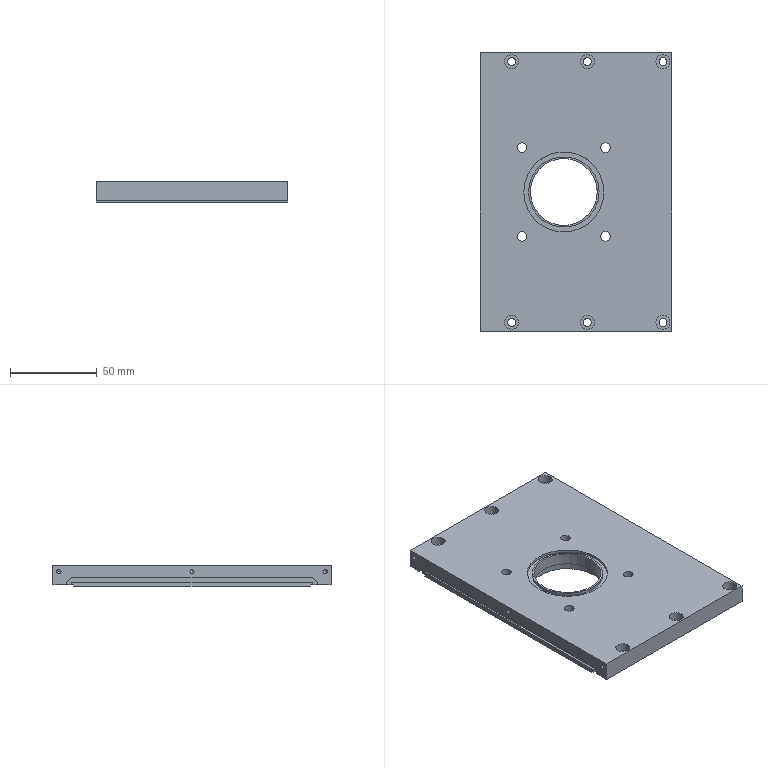NC program | NX | posted with a generic post | part box 110 x 160 x 12 mm
Lines 3477 to 4419 of 4419:
(PLANAR_MILL_COPY_COPY_COPY_COPY_COPY_COPY_1_COPY_1_COPY , TOOL : D6A45)
N6940 T01 M6
N6942 G54
N6944 G17 G0 G90 X-65.933 Y0.483 B0. C0. S9500 M3
N6946 G43 Z30. H1
N6948 Z0.84
N6950 G94 G1 X-66.061 Y0.254 Z0.77 F1250.
N6952 Y-0.254 Z0.634
N6954 X-65.771 Y-0.771 Z0.475
N6956 X-65.254 Y-1.061 Z0.316
N6958 X-64.746 Z0.18
N6960 X-64.229 Y-0.771 Z0.021
N6962 X-63.939 Y-0.254 Z-0.138
N6964 Y0.254 Z-0.274
N6966 X-64.229 Y0.771 Z-0.433
N6968 X-64.746 Y1.061 Z-0.592
N6970 X-65. Z-0.66
N6972 G3 X-66.061 Y0. R1.061
N6974 X-65. Y1.061 R-1.061
N6976 X-65.866 Y0.561 R1.
N6978 G1 Z0.84
N6980 G0 Z30.
N6982 X-44.318 Y1.717
N6984 Z0.84
N6986 G1 Z-0.66
N6988 X-44.134 Y2.44
N6990 G3 X-45. Y2.94 R1.
N6992 G1 X-45.5
N6994 G3 X-47.44 Y1. R1.94
N6996 X-45.5 Y-0.94 R1.94
N6998 G1 X-44.5
N7000 G3 X-42.56 Y1. R1.94
N7002 X-44.5 Y2.94 R1.94
N7004 G1 X-45.
N7006 G3 X-45.866 Y2.44 R1.
N7008 G1 X-45.682 Y1.717
N7010 Z0.84
N7012 G0 Z30.
N7014 X-0.933 Y0.483
N7016 Z0.84
N7018 G1 X-1.061 Y0.254 Z0.77
N7020 Y-0.254 Z0.634
N7022 X-0.771 Y-0.771 Z0.475
N7024 X-0.254 Y-1.061 Z0.316
N7026 X0.254 Z0.18
N7028 X0.771 Y-0.771 Z0.021
N7030 X1.061 Y-0.254 Z-0.138
N7032 Y0.254 Z-0.274
N7034 X0.771 Y0.771 Z-0.433
N7036 X0.254 Y1.061 Z-0.592
N7038 X0. Z-0.66
N7040 G3 X-1.061 Y0. R1.061
N7042 X0. Y1.061 R-1.061
N7044 X-0.866 Y0.561 R1.
N7046 G1 Z0.84
N7048 G0 Z30.
N7050 X45.381 Y1.634
N7052 Z0.84
N7054 G1 Z-0.66
N7056 X45.866 Y2.44
N7058 G3 X45. Y2.94 R1.
N7060 X43.06 Y1. R1.94
N7062 X45. Y2.94 R-1.94
N7064 X44.134 Y2.44 R1.
N7066 G1 X44.619 Y1.634
N7068 Z0.84
N7070 G0 Z30.
N7072 X64.067 Y0.483
N7074 Z0.84
N7076 G1 X63.939 Y0.254 Z0.77
N7078 Y-0.254 Z0.634
N7080 X64.229 Y-0.771 Z0.475
N7082 X64.746 Y-1.061 Z0.316
N7084 X65.254 Z0.18
N7086 X65.771 Y-0.771 Z0.021
N7088 X66.061 Y-0.254 Z-0.138
N7090 Y0.254 Z-0.274
N7092 X65.771 Y0.771 Z-0.433
N7094 X65.254 Y1.061 Z-0.592
N7096 X65. Z-0.66
N7098 G3 X63.939 Y0. R1.061
N7100 X65. Y1.061 R-1.061
N7102 X64.134 Y0.561 R1.
N7104 G1 Z0.84
N7106 G0 Z30.
N7108 M5
(刀补17 , TOOL : D3)
N7110 T17 M6
N7112 G54
N7114 G17 G0 G90 X-46.153 Y1.662 B0. C0. S9500 M3
N7116 G43 Z30. H17
N7118 Z1.
N7120 G94 G1 X-46.234 Y1.591 Z0.994 F1000.
N7122 X-46.392 Y1.304 Z0.977
N7124 X-46.442 Y0.98 Z0.96
N7126 X-46.379 Y0.659 Z0.943
N7128 X-46.209 Y0.379 Z0.926
N7130 X-46.001 Y0.201 Z0.911
N7132 X-45.826 Y0.115 Z0.901
N7134 X-45.637 Y0.067 Z0.891
N7136 X-44.363 Z0.824
N7138 X-44.105 Y0.144 Z0.81
N7140 X-43.879 Y0.291 Z0.796
N7142 X-43.704 Y0.496 Z0.782
N7144 X-43.592 Y0.746 Z0.767
N7146 X-43.559 Y1.063 Z0.751
N7148 X-43.634 Y1.372 Z0.734
N7150 X-43.808 Y1.64 Z0.717
N7152 X-44.06 Y1.834 Z0.701
N7154 X-44.363 Y1.933 Z0.684
N7156 X-45.637 Z0.617
N7158 X-45.735 Y1.913 Z0.612
N7160 X-45.987 Y1.807 Z0.598
N7162 X-46.234 Y1.591 Z0.58
N7164 X-46.392 Y1.304 Z0.563
N7166 X-46.442 Y0.98 Z0.546
N7168 X-46.379 Y0.659 Z0.529
N7170 X-46.209 Y0.379 Z0.512
N7172 X-46.001 Y0.201 Z0.497
N7174 X-45.826 Y0.115 Z0.487
N7176 X-45.637 Y0.067 Z0.477
N7178 X-44.363 Z0.41
N7180 X-44.105 Y0.144 Z0.396
N7182 X-43.879 Y0.291 Z0.382
N7184 X-43.704 Y0.496 Z0.368
N7186 X-43.592 Y0.746 Z0.354
N7188 X-43.559 Y1.063 Z0.337
N7190 X-43.634 Y1.372 Z0.32
N7192 X-43.808 Y1.64 Z0.303
N7194 X-44.06 Y1.834 Z0.287
N7196 X-44.363 Y1.933 Z0.27
N7198 X-45.637 Z0.203
N7200 X-45.735 Y1.913 Z0.198
N7202 X-45.987 Y1.807 Z0.184
N7204 X-46.234 Y1.591 Z0.166
N7206 X-46.392 Y1.304 Z0.149
N7208 X-46.442 Y0.98 Z0.132
N7210 X-46.379 Y0.659 Z0.115
N7212 X-46.209 Y0.379 Z0.098
N7214 X-46.001 Y0.201 Z0.083
N7216 X-45.826 Y0.115 Z0.073
N7218 X-45.637 Y0.067 Z0.063
N7220 X-44.363 Z-0.004
N7222 X-44.105 Y0.144 Z-0.018
N7224 X-43.879 Y0.291 Z-0.032
N7226 X-43.704 Y0.496 Z-0.046
N7228 X-43.592 Y0.746 Z-0.06
N7230 X-43.559 Y1.063 Z-0.077
N7232 X-43.634 Y1.372 Z-0.094
N7234 X-43.808 Y1.64 Z-0.111
N7236 X-44.06 Y1.834 Z-0.127
N7238 X-44.363 Y1.933 Z-0.144
N7240 X-45.637 Z-0.211
N7242 X-45.735 Y1.913 Z-0.216
N7244 X-45.987 Y1.807 Z-0.23
N7246 X-46.234 Y1.591 Z-0.247
N7248 X-46.392 Y1.304 Z-0.265
N7250 X-46.442 Y0.98 Z-0.282
N7252 X-46.379 Y0.659 Z-0.299
N7254 X-46.209 Y0.379 Z-0.316
N7256 X-46.001 Y0.201 Z-0.33
N7258 X-45.826 Y0.115 Z-0.341
N7260 X-45.637 Y0.067 Z-0.351
N7262 X-44.363 Z-0.418
N7264 X-44.105 Y0.144 Z-0.432
N7266 X-43.879 Y0.291 Z-0.446
N7268 X-43.704 Y0.496 Z-0.46
N7270 X-43.592 Y0.746 Z-0.474
N7272 X-43.559 Y1.063 Z-0.491
N7274 X-43.634 Y1.372 Z-0.508
N7276 X-43.808 Y1.64 Z-0.524
N7278 X-44.06 Y1.834 Z-0.541
N7280 X-44.363 Y1.933 Z-0.558
N7282 X-45.637 Z-0.625
N7284 X-45.735 Y1.913 Z-0.63
N7286 X-45.987 Y1.807 Z-0.644
N7288 X-46.234 Y1.591 Z-0.661
N7290 X-46.392 Y1.304 Z-0.679
N7292 X-46.442 Y0.98 Z-0.696
N7294 X-46.379 Y0.659 Z-0.713
N7296 X-46.209 Y0.379 Z-0.73
N7298 X-46.001 Y0.201 Z-0.744
N7300 X-45.826 Y0.115 Z-0.755
N7302 X-45.637 Y0.067 Z-0.765
N7304 X-44.363 Z-0.832
N7306 X-44.105 Y0.144 Z-0.846
N7308 X-43.879 Y0.291 Z-0.86
N7310 X-43.704 Y0.496 Z-0.874
N7312 X-43.592 Y0.746 Z-0.888
N7314 X-43.559 Y1.063 Z-0.905
N7316 X-43.634 Y1.372 Z-0.922
N7318 X-43.808 Y1.64 Z-0.938
N7320 X-44.06 Y1.834 Z-0.955
N7322 X-44.363 Y1.933 Z-0.972
N7324 X-44.902 Z-1.
N7326 G41 X-45. Y1.95 D17
N7328 X-45.5
N7330 G3 X-46.45 Y1. R0.95
N7332 X-45.5 Y0.05 R0.95
N7334 G1 X-44.5
N7336 G3 X-43.55 Y1. R0.95
N7338 X-44.5 Y1.95 R0.95
N7340 G1 X-45.
N7342 X-45.359 Z-1.06
N7344 X-45.478 Y1.946 Z-1.08
N7346 X-45.591 Y1.936 Z-1.099
N7348 X-45.67 Y1.928 Z-1.112
N7350 X-45.713 Y1.916 Z-1.12
N7352 X-45.829 Y1.885 Z-1.14
N7354 X-45.9 Y1.852 Z-1.153
N7356 X-45.935 Y1.835 Z-1.16
N7358 X-46.017 Y1.786 Z-1.176
N7360 X-46.082 Y1.741 Z-1.189
N7362 X-46.129 Y1.701 Z-1.2
N7364 X-46.196 Y1.635 Z-1.216
N7366 X-46.228 Y1.6 Z-1.224
N7368 X-46.283 Y1.521 Z-1.24
N7370 X-46.336 Y1.433 Z-1.257
N7372 X-46.37 Y1.361 Z-1.271
N7374 X-46.39 Y1.31 Z-1.28
N7376 X-46.425 Y1.183 Z-1.302
N7378 X-46.431 Y1.149 Z-1.308
N7380 X-46.438 Y1.079 Z-1.32
N7382 X-46.442 Y0.968 Z-1.339
N7384 X-46.435 Y0.889 Z-1.352
N7386 X-46.431 Y0.842 Z-1.36
N7388 X-46.41 Y0.762 Z-1.374
N7390 X-46.39 Y0.686 Z-1.387
N7392 X-46.359 Y0.617 Z-1.4
N7394 X-46.312 Y0.52 Z-1.418
N7396 X-46.267 Y0.455 Z-1.431
N7398 X-46.238 Y0.414 Z-1.44
N7400 X-46.176 Y0.345 Z-1.456
N7402 X-46.12 Y0.29 Z-1.469
N7404 X-46.068 Y0.25 Z-1.48
N7406 X-45.982 Y0.189 Z-1.498
N7408 X-45.912 Y0.154 Z-1.511
N7410 X-45.863 Y0.132 Z-1.52
N7412 X-45.778 Y0.1 Z-1.535
N7414 X-45.701 Y0.08 Z-1.549
N7416 X-45.636 Y0.068 Z-1.56
N7418 X-45.517 Y0.057 Z-1.58
N7420 X-45.398 Y0.05 Z-1.6
N7422 X-44.681 Z-1.72
N7424 X-44.562 Z-1.74
N7426 X-44.443 Y0.061 Z-1.76
N7428 X-44.328 Y0.073 Z-1.779
N7430 X-44.252 Y0.092 Z-1.793
N7432 X-44.21 Y0.104 Z-1.8
N7434 X-44.122 Y0.138 Z-1.816
N7436 X-44.051 Y0.172 Z-1.829
N7438 X-43.996 Y0.204 Z-1.84
N7440 X-43.917 Y0.259 Z-1.856
N7442 X-43.88 Y0.289 Z-1.864
N7444 X-43.815 Y0.355 Z-1.88
N7446 X-43.748 Y0.434 Z-1.897
N7448 X-43.703 Y0.499 Z-1.911
N7450 X-43.674 Y0.545 Z-1.92
N7452 X-43.621 Y0.658 Z-1.941
N7454 X-43.608 Y0.693 Z-1.947
N7456 X-43.589 Y0.766 Z-1.96
N7458 X-43.566 Y0.882 Z-1.98
N7460 X-43.55 Y1. Z-2.
N7462 G3 X-44.5 Y1.95 R0.95
N7464 G1 X-45.
N7466 X-45.359 Z-2.06
N7468 X-45.478 Y1.946 Z-2.08
N7470 X-45.596 Y1.936 Z-2.1
N7472 X-45.713 Y1.916 Z-2.12
N7474 X-45.803 Y1.893 Z-2.136
N7476 X-45.846 Y1.877 Z-2.143
N7478 X-45.935 Y1.835 Z-2.16
N7480 X-46.016 Y1.787 Z-2.176
N7482 X-46.081 Y1.742 Z-2.189
N7484 X-46.129 Y1.701 Z-2.2
N7486 X-46.197 Y1.633 Z-2.216
N7488 X-46.23 Y1.597 Z-2.224
N7490 X-46.283 Y1.521 Z-2.24
N7492 X-46.336 Y1.432 Z-2.257
N7494 X-46.369 Y1.361 Z-2.271
N7496 X-46.39 Y1.31 Z-2.28
N7498 X-46.414 Y1.226 Z-2.295
N7500 X-46.425 Y1.183 Z-2.302
N7502 X-46.431 Y1.149 Z-2.308
N7504 X-46.437 Y1.079 Z-2.32
N7506 X-46.442 Y0.968 Z-2.339
N7508 X-46.435 Y0.89 Z-2.352
N7510 X-46.43 Y0.842 Z-2.36
N7512 X-46.41 Y0.762 Z-2.374
N7514 X-46.39 Y0.686 Z-2.387
N7516 X-46.359 Y0.617 Z-2.4
N7518 X-46.312 Y0.52 Z-2.418
N7520 X-46.267 Y0.456 Z-2.431
N7522 X-46.238 Y0.414 Z-2.44
N7524 X-46.176 Y0.346 Z-2.455
N7526 X-46.121 Y0.29 Z-2.469
N7528 X-46.068 Y0.25 Z-2.48
N7530 X-45.983 Y0.189 Z-2.498
N7532 X-45.912 Y0.154 Z-2.511
N7534 X-45.863 Y0.132 Z-2.52
N7536 X-45.778 Y0.101 Z-2.535
N7538 X-45.702 Y0.081 Z-2.549
N7540 X-45.636 Y0.068 Z-2.56
N7542 X-45.517 Y0.057 Z-2.58
N7544 X-45.398 Y0.05 Z-2.6
N7546 X-44.681 Z-2.72
N7548 X-44.562 Y0.051 Z-2.74
N7550 X-44.443 Y0.061 Z-2.76
N7552 X-44.328 Y0.073 Z-2.779
N7554 X-44.252 Y0.093 Z-2.793
N7556 X-44.21 Y0.104 Z-2.8
N7558 X-44.123 Y0.138 Z-2.816
N7560 X-44.051 Y0.171 Z-2.829
N7562 X-43.996 Y0.204 Z-2.84
N7564 X-43.918 Y0.259 Z-2.856
N7566 X-43.881 Y0.289 Z-2.864
N7568 X-43.815 Y0.355 Z-2.88
N7570 X-43.748 Y0.434 Z-2.897
N7572 X-43.703 Y0.498 Z-2.911
N7574 X-43.674 Y0.545 Z-2.92
N7576 X-43.621 Y0.661 Z-2.942
N7578 X-43.608 Y0.695 Z-2.948
N7580 X-43.589 Y0.766 Z-2.96
N7582 X-43.566 Y0.882 Z-2.98
N7584 X-43.55 Y1. Z-3.
N7586 G3 X-44.5 Y1.95 R0.95
N7588 G1 X-45.
N7590 X-45.359 Z-3.06
N7592 X-45.478 Y1.946 Z-3.08
N7594 X-45.596 Y1.936 Z-3.1
N7596 X-45.713 Y1.916 Z-3.12
N7598 X-45.802 Y1.893 Z-3.135
N7600 X-45.845 Y1.877 Z-3.143
N7602 X-45.875 Y1.863 Z-3.149
N7604 X-45.935 Y1.835 Z-3.16
N7606 X-46.017 Y1.786 Z-3.176
N7608 X-46.081 Y1.741 Z-3.189
N7610 X-46.129 Y1.7 Z-3.2
N7612 X-46.197 Y1.633 Z-3.216
N7614 X-46.229 Y1.598 Z-3.224
N7616 X-46.248 Y1.573 Z-3.229
N7618 X-46.283 Y1.521 Z-3.24
N7620 X-46.337 Y1.431 Z-3.258
N7622 X-46.37 Y1.359 Z-3.271
N7624 X-46.39 Y1.31 Z-3.28
N7626 X-46.413 Y1.226 Z-3.295
N7628 X-46.425 Y1.184 Z-3.302
N7630 X-46.431 Y1.149 Z-3.308
N7632 X-46.437 Y1.079 Z-3.32
N7634 X-46.441 Y0.969 Z-3.338
N7636 X-46.435 Y0.891 Z-3.352
N7638 X-46.43 Y0.842 Z-3.36
N7640 X-46.41 Y0.763 Z-3.374
N7642 X-46.39 Y0.687 Z-3.387
N7644 X-46.359 Y0.617 Z-3.4
N7646 X-46.313 Y0.521 Z-3.418
N7648 X-46.267 Y0.456 Z-3.431
N7650 X-46.237 Y0.414 Z-3.44
N7652 X-46.177 Y0.347 Z-3.455
N7654 X-46.121 Y0.291 Z-3.469
N7656 X-46.068 Y0.25 Z-3.48
N7658 X-45.983 Y0.19 Z-3.497
N7660 X-45.913 Y0.155 Z-3.511
N7662 X-45.863 Y0.132 Z-3.52
N7664 X-45.779 Y0.101 Z-3.535
N7666 X-45.703 Y0.081 Z-3.548
N7668 X-45.636 Y0.068 Z-3.56
N7670 X-45.517 Y0.057 Z-3.58
N7672 X-45.398 Y0.05 Z-3.6
N7674 X-44.681 Z-3.72
N7676 X-44.562 Y0.051 Z-3.74
N7678 X-44.443 Y0.061 Z-3.76
N7680 X-44.328 Y0.072 Z-3.779
N7682 X-44.252 Y0.093 Z-3.793
N7684 X-44.211 Y0.104 Z-3.8
N7686 X-44.123 Y0.138 Z-3.816
N7688 X-44.052 Y0.171 Z-3.829
N7690 X-43.997 Y0.204 Z-3.84
N7692 X-43.919 Y0.259 Z-3.856
N7694 X-43.882 Y0.288 Z-3.864
N7696 X-43.815 Y0.355 Z-3.88
N7698 X-43.749 Y0.434 Z-3.897
N7700 X-43.703 Y0.498 Z-3.911
N7702 X-43.674 Y0.545 Z-3.92
N7704 X-43.638 Y0.622 Z-3.934
N7706 X-43.608 Y0.695 Z-3.948
N7708 X-43.589 Y0.766 Z-3.96
N7710 X-43.566 Y0.882 Z-3.98
N7712 X-43.55 Y1. Z-4.
N7714 G3 X-44.5 Y1.95 R0.95
N7716 G1 X-45.
N7718 X-45.359 Z-4.06
N7720 X-45.478 Y1.945 Z-4.08
N7722 X-45.596 Y1.936 Z-4.1
N7724 X-45.713 Y1.916 Z-4.12
N7726 X-45.802 Y1.893 Z-4.135
N7728 X-45.845 Y1.877 Z-4.143
N7730 X-45.935 Y1.835 Z-4.16
N7732 X-46.017 Y1.786 Z-4.176
N7734 X-46.081 Y1.741 Z-4.189
N7736 X-46.129 Y1.7 Z-4.2
N7738 X-46.196 Y1.633 Z-4.216
N7740 X-46.228 Y1.598 Z-4.224
N7742 X-46.247 Y1.573 Z-4.229
N7744 X-46.283 Y1.521 Z-4.24
N7746 X-46.336 Y1.431 Z-4.258
N7748 X-46.37 Y1.36 Z-4.271
N7750 X-46.39 Y1.31 Z-4.28
N7752 X-46.413 Y1.227 Z-4.295
N7754 X-46.424 Y1.185 Z-4.302
N7756 X-46.431 Y1.15 Z-4.308
N7758 X-46.437 Y1.079 Z-4.32
N7760 X-46.441 Y0.97 Z-4.338
N7762 X-46.434 Y0.891 Z-4.352
N7764 X-46.43 Y0.842 Z-4.36
N7766 X-46.41 Y0.764 Z-4.374
N7768 X-46.39 Y0.687 Z-4.387
N7770 X-46.359 Y0.617 Z-4.4
N7772 X-46.313 Y0.521 Z-4.418
N7774 X-46.267 Y0.457 Z-4.431
N7776 X-46.237 Y0.415 Z-4.44
N7778 X-46.177 Y0.347 Z-4.455
N7780 X-46.121 Y0.291 Z-4.469
N7782 X-46.068 Y0.25 Z-4.48
N7784 X-45.984 Y0.19 Z-4.497
N7786 X-45.913 Y0.155 Z-4.511
N7788 X-45.863 Y0.132 Z-4.52
N7790 X-45.78 Y0.101 Z-4.535
N7792 X-45.704 Y0.081 Z-4.548
N7794 X-45.636 Y0.068 Z-4.56
N7796 X-45.517 Y0.057 Z-4.58
N7798 X-45.398 Y0.05 Z-4.6
N7800 X-44.681 Z-4.72
N7802 X-44.562 Y0.051 Z-4.74
N7804 X-44.443 Y0.061 Z-4.76
N7806 X-44.328 Y0.073 Z-4.779
N7808 X-44.252 Y0.093 Z-4.793
N7810 X-44.211 Y0.104 Z-4.8
N7812 X-44.122 Y0.139 Z-4.816
N7814 X-44.05 Y0.172 Z-4.829
N7816 X-43.997 Y0.204 Z-4.84
N7818 X-43.917 Y0.261 Z-4.856
N7820 X-43.879 Y0.291 Z-4.865
N7822 X-43.857 Y0.312 Z-4.87
N7824 X-43.815 Y0.356 Z-4.88
N7826 X-43.748 Y0.435 Z-4.898
N7828 X-43.702 Y0.5 Z-4.911
N7830 X-43.674 Y0.545 Z-4.92
N7832 X-43.639 Y0.621 Z-4.934
N7834 X-43.621 Y0.66 Z-4.941
N7836 X-43.609 Y0.694 Z-4.948
N7838 X-43.589 Y0.766 Z-4.96
N7840 X-43.566 Y0.883 Z-4.98
N7842 X-43.55 Y1. Z-5.
N7844 G3 X-44.5 Y1.95 R0.95
N7846 G1 X-45.
N7848 X-45.359 Z-5.06
N7850 X-45.478 Y1.945 Z-5.08
N7852 X-45.596 Y1.935 Z-5.1
N7854 X-45.713 Y1.916 Z-5.12
N7856 X-45.802 Y1.893 Z-5.135
N7858 X-45.845 Y1.877 Z-5.143
N7860 X-45.935 Y1.835 Z-5.16
N7862 X-46.017 Y1.786 Z-5.176
N7864 X-46.081 Y1.741 Z-5.189
N7866 X-46.129 Y1.7 Z-5.2
N7868 X-46.196 Y1.633 Z-5.216
N7870 X-46.229 Y1.599 Z-5.224
N7872 X-46.283 Y1.521 Z-5.24
N7874 X-46.336 Y1.431 Z-5.258
N7876 X-46.37 Y1.36 Z-5.271
N7878 X-46.39 Y1.31 Z-5.28
N7880 X-46.414 Y1.225 Z-5.295
N7882 X-46.425 Y1.182 Z-5.302
N7884 X-46.431 Y1.148 Z-5.308
N7886 X-46.437 Y1.079 Z-5.32
N7888 X-46.441 Y0.967 Z-5.339
N7890 X-46.434 Y0.889 Z-5.352
N7892 X-46.43 Y0.842 Z-5.36
N7894 X-46.41 Y0.764 Z-5.374
N7896 X-46.39 Y0.688 Z-5.387
N7898 X-46.359 Y0.617 Z-5.4
N7900 X-46.313 Y0.522 Z-5.418
N7902 X-46.268 Y0.457 Z-5.431
N7904 X-46.237 Y0.415 Z-5.44
N7906 X-46.175 Y0.346 Z-5.456
N7908 X-46.119 Y0.29 Z-5.469
N7910 X-46.068 Y0.25 Z-5.48
N7912 X-45.984 Y0.191 Z-5.497
N7914 X-45.913 Y0.156 Z-5.511
N7916 X-45.863 Y0.133 Z-5.52
N7918 X-45.78 Y0.102 Z-5.535
N7920 X-45.704 Y0.081 Z-5.548
N7922 X-45.636 Y0.069 Z-5.56
N7924 X-45.517 Y0.058 Z-5.58
N7926 X-45.398 Y0.05 Z-5.6
N7928 X-44.681 Z-5.72
N7930 X-44.562 Y0.051 Z-5.74
N7932 X-44.443 Y0.061 Z-5.76
N7934 X-44.328 Y0.073 Z-5.779
N7936 X-44.252 Y0.093 Z-5.793
N7938 X-44.211 Y0.104 Z-5.8
N7940 X-44.122 Y0.138 Z-5.816
N7942 X-44.051 Y0.172 Z-5.829
N7944 X-43.997 Y0.205 Z-5.84
N7946 X-43.918 Y0.261 Z-5.856
N7948 X-43.88 Y0.291 Z-5.865
N7950 X-43.858 Y0.312 Z-5.87
N7952 X-43.815 Y0.356 Z-5.88
N7954 X-43.748 Y0.435 Z-5.897
N7956 X-43.703 Y0.499 Z-5.911
N7958 X-43.675 Y0.546 Z-5.92
N7960 X-43.639 Y0.621 Z-5.934
N7962 X-43.621 Y0.659 Z-5.941
N7964 X-43.609 Y0.694 Z-5.947
N7966 X-43.589 Y0.766 Z-5.96
N7968 X-43.567 Y0.883 Z-5.98
N7970 X-43.55 Y1. Z-6.
N7972 G3 X-44.5 Y1.95 R0.95
N7974 G1 X-45.5
N7976 G3 X-46.45 Y1. R0.95
N7978 X-45.5 Y0.05 R0.95
N7980 G1 X-44.5
N7982 G3 X-43.55 Y1. R0.95
N7984 G40
N7986 G1 X-43.567 Y1.098
N7988 Z-5.
N7990 G0 Z30.
N7992 X45.252 Y0.094
N7994 Z1.
N7996 G1 X45.552 Y0.229 Z0.983
N7998 X45.807 Y0.502 Z0.963
N8000 X45.915 Y0.755 Z0.949
N8002 X45.948 Y0.987 Z0.937
N8004 X45.912 Y1.259 Z0.922
N8006 X45.769 Y1.554 Z0.905
N8008 X45.534 Y1.783 Z0.888
N8010 X45.235 Y1.918 Z0.871
N8012 X45.049 Y1.938 Z0.861
N8014 X44.863 Z0.851
N8016 X44.758 Y1.916 Z0.845
N8018 X44.505 Y1.808 Z0.831
N8020 X44.26 Y1.592 Z0.814
N8022 X44.103 Y1.305 Z0.797
N8024 X44.052 Y0.982 Z0.78
N8026 X44.115 Y0.661 Z0.762
N8028 X44.283 Y0.38 Z0.745
N8030 X44.49 Y0.201 Z0.731
N8032 X44.839 Y0.066 Z0.711
N8034 X45.212 Y0.076 Z0.692
N8036 X45.552 Y0.229 Z0.672
N8038 X45.807 Y0.502 Z0.653
N8040 X45.915 Y0.755 Z0.638
N8042 X45.948 Y0.987 Z0.626
N8044 X45.912 Y1.259 Z0.612
N8046 X45.769 Y1.554 Z0.594
N8048 X45.534 Y1.783 Z0.577
N8050 X45.235 Y1.918 Z0.56
N8052 X45.049 Y1.938 Z0.55
N8054 X44.863 Z0.54
N8056 X44.758 Y1.916 Z0.535
N8058 X44.505 Y1.808 Z0.52
N8060 X44.26 Y1.592 Z0.503
N8062 X44.103 Y1.305 Z0.486
N8064 X44.052 Y0.982 Z0.469
N8066 X44.115 Y0.661 Z0.452
N8068 X44.283 Y0.38 Z0.435
N8070 X44.49 Y0.201 Z0.42
N8072 X44.839 Y0.066 Z0.401
N8074 X45.212 Y0.076 Z0.381
N8076 X45.552 Y0.229 Z0.362
N8078 X45.807 Y0.502 Z0.342
N8080 X45.915 Y0.755 Z0.328
N8082 X45.948 Y0.987 Z0.315
N8084 X45.912 Y1.259 Z0.301
N8086 X45.769 Y1.554 Z0.284
N8088 X45.534 Y1.783 Z0.267
N8090 X45.235 Y1.918 Z0.249
N8092 X45.049 Y1.938 Z0.24
N8094 X44.863 Z0.23
N8096 X44.758 Y1.916 Z0.224
N8098 X44.505 Y1.808 Z0.21
N8100 X44.26 Y1.592 Z0.193
N8102 X44.103 Y1.305 Z0.176
N8104 X44.052 Y0.982 Z0.158
N8106 X44.115 Y0.661 Z0.141
N8108 X44.283 Y0.38 Z0.124
N8110 X44.49 Y0.201 Z0.11
N8112 X44.839 Y0.066 Z0.09
N8114 X45.212 Y0.076 Z0.071
N8116 X45.552 Y0.229 Z0.051
N8118 X45.807 Y0.502 Z0.032
N8120 X45.915 Y0.755 Z0.017
N8122 X45.948 Y0.987 Z0.005
N8124 X45.912 Y1.259 Z-0.01
N8126 X45.769 Y1.554 Z-0.027
N8128 X45.534 Y1.783 Z-0.044
N8130 X45.235 Y1.918 Z-0.061
N8132 X45.049 Y1.938 Z-0.071
N8134 X44.863 Z-0.081
N8136 X44.758 Y1.916 Z-0.086
N8138 X44.505 Y1.808 Z-0.101
N8140 X44.26 Y1.592 Z-0.118
N8142 X44.103 Y1.305 Z-0.135
N8144 X44.052 Y0.982 Z-0.152
N8146 X44.115 Y0.661 Z-0.169
N8148 X44.283 Y0.38 Z-0.186
N8150 X44.49 Y0.201 Z-0.201
N8152 X44.839 Y0.066 Z-0.22
N8154 X45.212 Y0.076 Z-0.24
N8156 X45.552 Y0.229 Z-0.259
N8158 X45.807 Y0.502 Z-0.279
N8160 X45.915 Y0.755 Z-0.293
N8162 X45.948 Y0.987 Z-0.306
N8164 X45.912 Y1.259 Z-0.32
N8166 X45.769 Y1.554 Z-0.337
N8168 X45.534 Y1.783 Z-0.354
N8170 X45.235 Y1.918 Z-0.372
N8172 X45.049 Y1.938 Z-0.381
N8174 X44.863 Z-0.391
N8176 X44.758 Y1.916 Z-0.397
N8178 X44.505 Y1.808 Z-0.411
N8180 X44.26 Y1.592 Z-0.428
N8182 X44.103 Y1.305 Z-0.446
N8184 X44.052 Y0.982 Z-0.463
N8186 X44.115 Y0.661 Z-0.48
N8188 X44.283 Y0.38 Z-0.497
N8190 X44.49 Y0.201 Z-0.511
N8192 X44.839 Y0.066 Z-0.531
N8194 X45.212 Y0.076 Z-0.55
N8196 X45.552 Y0.229 Z-0.57
N8198 X45.807 Y0.502 Z-0.59
N8200 X45.915 Y0.755 Z-0.604
N8202 X45.948 Y0.987 Z-0.616
N8204 X45.912 Y1.259 Z-0.631
N8206 X45.769 Y1.554 Z-0.648
N8208 X45.534 Y1.783 Z-0.665
N8210 X45.235 Y1.918 Z-0.682
N8212 X45.049 Y1.938 Z-0.692
N8214 X44.863 Z-0.702
N8216 X44.758 Y1.916 Z-0.707
N8218 X44.505 Y1.808 Z-0.722
N8220 X44.26 Y1.592 Z-0.739
N8222 X44.103 Y1.305 Z-0.756
N8224 X44.052 Y0.982 Z-0.773
N8226 X44.115 Y0.661 Z-0.79
N8228 X44.283 Y0.38 Z-0.808
N8230 X44.49 Y0.201 Z-0.822
N8232 X44.839 Y0.066 Z-0.841
N8234 X45.212 Y0.076 Z-0.861
N8236 X45.552 Y0.229 Z-0.881
N8238 X45.807 Y0.502 Z-0.9
N8240 X45.915 Y0.755 Z-0.915
N8242 X45.948 Y0.987 Z-0.927
N8244 X45.912 Y1.259 Z-0.941
N8246 X45.769 Y1.554 Z-0.958
N8248 X45.534 Y1.783 Z-0.976
N8250 X45.235 Y1.918 Z-0.993
N8252 X45.098 Y1.933 Z-1.
N8254 G41 X45. Y1.95
N8256 G3 X44.05 Y1. R0.95
N8258 X45. Y1.95 R-0.95
N8260 G1 X44.909 Y1.936 Z-1.021
N8262 X44.827 Y1.928 Z-1.039
N8264 X44.756 Y1.909 Z-1.056
N8266 X44.646 Y1.873 Z-1.082
N8268 X44.571 Y1.838 Z-1.1
N8270 X44.528 Y1.817 Z-1.111
N8272 X44.457 Y1.768 Z-1.131
N8274 X44.39 Y1.721 Z-1.149
N8276 X44.335 Y1.665 Z-1.167
N8278 X44.257 Y1.579 Z-1.193
N8280 X44.21 Y1.512 Z-1.211
N8282 X44.183 Y1.472 Z-1.222
N8284 X44.146 Y1.394 Z-1.242
N8286 X44.111 Y1.319 Z-1.26
N8288 X44.091 Y1.244 Z-1.278
N8290 X44.067 Y1.13 Z-1.304
N8292 X44.06 Y1.048 Z-1.322
N8294 X44.056 Y1. Z-1.333
N8296 X44.064 Y0.914 Z-1.353
N8298 X44.071 Y0.832 Z-1.371
N8300 X44.091 Y0.756 Z-1.389
N8302 X44.127 Y0.646 Z-1.415
N8304 X44.162 Y0.572 Z-1.433
N8306 X44.183 Y0.528 Z-1.444
N8308 X44.232 Y0.457 Z-1.464
N8310 X44.279 Y0.39 Z-1.482
N8312 X44.335 Y0.335 Z-1.5
N8314 X44.421 Y0.257 Z-1.526
N8316 X44.488 Y0.21 Z-1.545
N8318 X44.528 Y0.183 Z-1.556
N8320 X44.606 Y0.146 Z-1.575
N8322 X44.681 Y0.111 Z-1.594
N8324 X44.756 Y0.091 Z-1.611
N8326 X44.87 Y0.067 Z-1.637
N8328 X44.952 Y0.06 Z-1.656
N8330 X45. Y0.056 Z-1.667
N8332 X45.086 Y0.064 Z-1.686
N8334 X45.168 Y0.071 Z-1.705
N8336 X45.244 Y0.091 Z-1.722
N8338 X45.354 Y0.127 Z-1.748
N8340 X45.428 Y0.162 Z-1.767
N8342 X45.472 Y0.183 Z-1.778
N8344 X45.543 Y0.232 Z-1.797
N8346 X45.61 Y0.279 Z-1.816
N8348 X45.665 Y0.335 Z-1.833
N8350 X45.743 Y0.421 Z-1.859
N8352 X45.79 Y0.488 Z-1.878
N8354 X45.817 Y0.528 Z-1.889
N8356 X45.852 Y0.602 Z-1.907
N8358 X45.887 Y0.676 Z-1.926
N8360 X45.909 Y0.757 Z-1.944
N8362 X45.934 Y0.878 Z-1.972
N8364 X45.95 Y1. Z-2.
N8366 G3 X45. Y1.95 R0.95
N8368 G1 X44.909 Y1.936 Z-2.021
N8370 X44.827 Y1.928 Z-2.039
N8372 X44.757 Y1.909 Z-2.056
N8374 X44.646 Y1.873 Z-2.082
N8376 X44.572 Y1.838 Z-2.1
N8378 X44.528 Y1.817 Z-2.111
N8380 X44.458 Y1.768 Z-2.13
N8382 X44.39 Y1.721 Z-2.149
N8384 X44.335 Y1.665 Z-2.167
N8386 X44.257 Y1.579 Z-2.193
N8388 X44.21 Y1.512 Z-2.211
N8390 X44.183 Y1.472 Z-2.222
N8392 X44.146 Y1.394 Z-2.242
N8394 X44.112 Y1.319 Z-2.26
N8396 X44.091 Y1.243 Z-2.278
N8398 X44.067 Y1.13 Z-2.304
N8400 X44.06 Y1.049 Z-2.322
N8402 X44.056 Y1. Z-2.333
N8404 X44.064 Y0.914 Z-2.353
N8406 X44.071 Y0.833 Z-2.371
N8408 X44.091 Y0.757 Z-2.389
N8410 X44.127 Y0.646 Z-2.415
N8412 X44.162 Y0.572 Z-2.433
N8414 X44.183 Y0.528 Z-2.444
N8416 X44.232 Y0.458 Z-2.464
N8418 X44.279 Y0.391 Z-2.482
N8420 X44.335 Y0.335 Z-2.5
N8422 X44.421 Y0.257 Z-2.526
N8424 X44.488 Y0.21 Z-2.544
N8426 X44.528 Y0.183 Z-2.556
N8428 X44.606 Y0.146 Z-2.575
N8430 X44.68 Y0.112 Z-2.593
N8432 X44.757 Y0.091 Z-2.611
N8434 X44.87 Y0.067 Z-2.637
N8436 X44.951 Y0.06 Z-2.656
N8438 X45. Y0.056 Z-2.667
N8440 X45.085 Y0.064 Z-2.686
N8442 X45.167 Y0.071 Z-2.705
N8444 X45.243 Y0.091 Z-2.722
N8446 X45.354 Y0.127 Z-2.748
N8448 X45.428 Y0.162 Z-2.767
N8450 X45.472 Y0.183 Z-2.778
N8452 X45.542 Y0.232 Z-2.797
N8454 X45.609 Y0.279 Z-2.816
N8456 X45.665 Y0.335 Z-2.833
N8458 X45.743 Y0.421 Z-2.859
N8460 X45.789 Y0.488 Z-2.878
N8462 X45.817 Y0.528 Z-2.889
N8464 X45.852 Y0.601 Z-2.907
N8466 X45.886 Y0.676 Z-2.926
N8468 X45.909 Y0.757 Z-2.944
N8470 X45.933 Y0.878 Z-2.972
N8472 X45.95 Y1. Z-3.
N8474 G3 X45. Y1.95 R0.95
N8476 G1 X44.909 Y1.937 Z-3.021
N8478 X44.827 Y1.927 Z-3.039
N8480 X44.757 Y1.909 Z-3.056
N8482 X44.646 Y1.873 Z-3.081
N8484 X44.572 Y1.838 Z-3.1
N8486 X44.528 Y1.817 Z-3.111
N8488 X44.458 Y1.768 Z-3.13
N8490 X44.391 Y1.721 Z-3.149
N8492 X44.335 Y1.665 Z-3.167
N8494 X44.257 Y1.58 Z-3.193
N8496 X44.211 Y1.512 Z-3.211
N8498 X44.183 Y1.472 Z-3.222
N8500 X44.147 Y1.394 Z-3.241
N8502 X44.112 Y1.32 Z-3.26
N8504 X44.091 Y1.243 Z-3.278
N8506 X44.067 Y1.131 Z-3.304
N8508 X44.06 Y1.049 Z-3.322
N8510 X44.056 Y1. Z-3.333
N8512 X44.064 Y0.915 Z-3.353
N8514 X44.071 Y0.833 Z-3.371
N8516 X44.091 Y0.757 Z-3.389
N8518 X44.127 Y0.647 Z-3.415
N8520 X44.162 Y0.573 Z-3.433
N8522 X44.183 Y0.528 Z-3.444
N8524 X44.232 Y0.458 Z-3.464
N8526 X44.279 Y0.391 Z-3.482
N8528 X44.335 Y0.335 Z-3.5
N8530 X44.42 Y0.258 Z-3.526
N8532 X44.488 Y0.211 Z-3.544
N8534 X44.528 Y0.183 Z-3.556
N8536 X44.605 Y0.147 Z-3.575
N8538 X44.68 Y0.112 Z-3.593
N8540 X44.757 Y0.091 Z-3.611
N8542 X44.869 Y0.067 Z-3.637
N8544 X44.951 Y0.06 Z-3.655
N8546 X45. Y0.057 Z-3.667
N8548 X45.085 Y0.064 Z-3.686
N8550 X45.167 Y0.071 Z-3.704
N8552 X45.243 Y0.091 Z-3.722
N8554 X45.353 Y0.127 Z-3.748
N8556 X45.427 Y0.162 Z-3.767
N8558 X45.472 Y0.183 Z-3.778
N8560 X45.541 Y0.232 Z-3.797
N8562 X45.609 Y0.279 Z-3.815
N8564 X45.665 Y0.335 Z-3.833
N8566 X45.742 Y0.42 Z-3.859
N8568 X45.789 Y0.487 Z-3.878
N8570 X45.817 Y0.528 Z-3.889
N8572 X45.851 Y0.601 Z-3.907
N8574 X45.886 Y0.675 Z-3.926
N8576 X45.908 Y0.757 Z-3.944
N8578 X45.933 Y0.878 Z-3.972
N8580 X45.95 Y1. Z-4.
N8582 G3 X45. Y1.95 R0.95
N8584 G1 X44.864 Y1.932 Z-4.031
N8586 X44.827 Y1.927 Z-4.039
N8588 X44.757 Y1.908 Z-4.056
N8590 X44.647 Y1.873 Z-4.081
N8592 X44.573 Y1.838 Z-4.1
N8594 X44.528 Y1.817 Z-4.111
N8596 X44.459 Y1.768 Z-4.13
N8598 X44.391 Y1.721 Z-4.149
N8600 X44.335 Y1.665 Z-4.167
N8602 X44.258 Y1.58 Z-4.192
N8604 X44.211 Y1.513 Z-4.211
N8606 X44.183 Y1.472 Z-4.222
N8608 X44.147 Y1.395 Z-4.241
N8610 X44.112 Y1.32 Z-4.26
N8612 X44.092 Y1.243 Z-4.278
N8614 X44.067 Y1.131 Z-4.304
N8616 X44.061 Y1.05 Z-4.322
N8618 X44.057 Y1. Z-4.333
N8620 X44.064 Y0.916 Z-4.352
N8622 X44.071 Y0.834 Z-4.371
N8624 X44.092 Y0.757 Z-4.389
N8626 X44.127 Y0.647 Z-4.415
N8628 X44.162 Y0.573 Z-4.433
N8630 X44.183 Y0.528 Z-4.444
N8632 X44.231 Y0.458 Z-4.464
N8634 X44.279 Y0.392 Z-4.482
N8636 X44.335 Y0.335 Z-4.5
N8638 X44.42 Y0.258 Z-4.526
N8640 X44.487 Y0.211 Z-4.544
N8642 X44.528 Y0.183 Z-4.556
N8644 X44.605 Y0.146 Z-4.575
N8646 X44.68 Y0.113 Z-4.593
N8648 X44.757 Y0.092 Z-4.611
N8650 X44.869 Y0.068 Z-4.637
N8652 X44.95 Y0.061 Z-4.655
N8654 X45. Y0.057 Z-4.667
N8656 X45.084 Y0.063 Z-4.686
N8658 X45.166 Y0.071 Z-4.704
N8660 X45.243 Y0.092 Z-4.722
N8662 X45.352 Y0.127 Z-4.748
N8664 X45.427 Y0.162 Z-4.766
N8666 X45.472 Y0.183 Z-4.778
N8668 X45.542 Y0.231 Z-4.797
N8670 X45.609 Y0.278 Z-4.815
N8672 X45.665 Y0.335 Z-4.833
N8674 X45.743 Y0.422 Z-4.86
N8676 X45.79 Y0.489 Z-4.878
N8678 X45.817 Y0.528 Z-4.889
N8680 X45.851 Y0.6 Z-4.907
N8682 X45.886 Y0.675 Z-4.925
N8684 X45.908 Y0.757 Z-4.944
N8686 X45.933 Y0.878 Z-4.972
N8688 X45.95 Y1. Z-5.
N8690 G3 X45. Y1.95 R0.95
N8692 G1 X44.91 Y1.936 Z-5.021
N8694 X44.828 Y1.928 Z-5.039
N8696 X44.757 Y1.908 Z-5.056
N8698 X44.646 Y1.872 Z-5.082
N8700 X44.571 Y1.837 Z-5.1
N8702 X44.528 Y1.817 Z-5.111
N8704 X44.459 Y1.769 Z-5.13
N8706 X44.392 Y1.722 Z-5.149
N8708 X44.335 Y1.665 Z-5.167
N8710 X44.257 Y1.578 Z-5.193
N8712 X44.21 Y1.511 Z-5.211
N8714 X44.183 Y1.472 Z-5.222
N8716 X44.147 Y1.395 Z-5.241
N8718 X44.112 Y1.321 Z-5.26
N8720 X44.092 Y1.243 Z-5.278
N8722 X44.068 Y1.129 Z-5.304
N8724 X44.061 Y1.048 Z-5.322
N8726 X44.057 Y1. Z-5.333
N8728 X44.063 Y0.916 Z-5.352
N8730 X44.071 Y0.834 Z-5.371
N8732 X44.092 Y0.757 Z-5.389
N8734 X44.128 Y0.646 Z-5.415
N8736 X44.163 Y0.572 Z-5.434
N8738 X44.183 Y0.528 Z-5.444
N8740 X44.231 Y0.459 Z-5.463
N8742 X44.278 Y0.392 Z-5.482
N8744 X44.335 Y0.335 Z-5.5
N8746 X44.422 Y0.257 Z-5.526
N8748 X44.489 Y0.211 Z-5.545
N8750 X44.528 Y0.183 Z-5.556
N8752 X44.604 Y0.147 Z-5.575
N8754 X44.679 Y0.112 Z-5.593
N8756 X44.757 Y0.092 Z-5.611
N8758 X44.871 Y0.068 Z-5.637
N8760 X44.952 Y0.061 Z-5.656
N8762 X45. Y0.057 Z-5.667
N8764 X45.084 Y0.063 Z-5.686
N8766 X45.166 Y0.071 Z-5.704
N8768 X45.243 Y0.092 Z-5.722
N8770 X45.354 Y0.128 Z-5.748
N8772 X45.428 Y0.163 Z-5.767
N8774 X45.472 Y0.183 Z-5.778
N8776 X45.541 Y0.231 Z-5.797
N8778 X45.608 Y0.278 Z-5.815
N8780 X45.665 Y0.335 Z-5.833
N8782 X45.743 Y0.422 Z-5.859
N8784 X45.789 Y0.489 Z-5.878
N8786 X45.817 Y0.528 Z-5.889
N8788 X45.851 Y0.6 Z-5.907
N8790 X45.886 Y0.674 Z-5.925
N8792 X45.908 Y0.757 Z-5.944
N8794 X45.933 Y0.878 Z-5.972
N8796 X45.95 Y1. Z-6.
N8798 G3 X45. Y1.95 R0.95
N8800 X45.95 Y1. R-0.95
N8802 G40
N8804 G1 X45.933 Y1.098
N8806 Z-5.
N8808 G0 Z30.
N8810 M5
N8812 M2